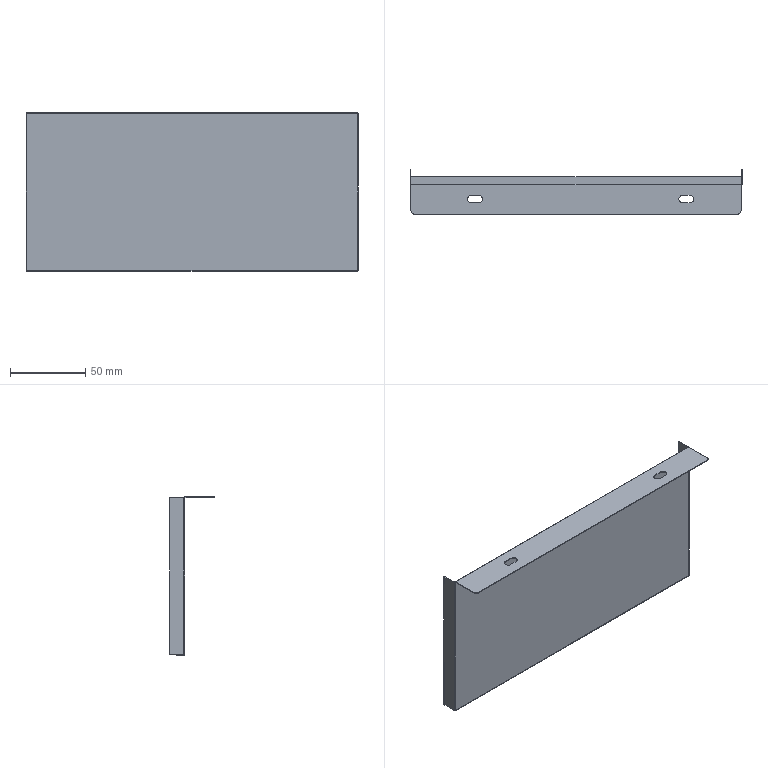Part | SolidWorks | features EdgeFlange 1, Fillet 1, FlatPattern 1, ICE 1, SMBaseFlange 1, SheetMetal 1 | 1 solid | 48 faces | box 220 x 29.5 x 105 mm | volume 15122 mm3 | plane 30 | cylinder 14 | spline 4 | commonest cylinder face diameters 5 x6 0.2 x4 1.2 x4
STEP:
#1=CARTESIAN_POINT('',(0.6,-0.5,0.6));
#2=VERTEX_POINT('',#1);
#3=CARTESIAN_POINT('',(219.4,-0.5,0.6));
#4=VERTEX_POINT('',#3);
#5=CARTESIAN_POINT('',(0.5707,-0.5,0.6));
#6=DIRECTION('',(1.,0.,0.));
#7=VECTOR('',#6,1000.);
#8=LINE('',#5,#7);
#9=EDGE_CURVE('',#2,#4,#8,.T.);
#10=ORIENTED_EDGE('',*,*,#9,.T.);
#11=CARTESIAN_POINT('',(219.4,-0.5,104.4));
#12=VERTEX_POINT('',#11);
#13=CARTESIAN_POINT('',(219.4,-0.5,0.5707));
#14=DIRECTION('',(0.,0.,1.));
#15=VECTOR('',#14,1000.);
#16=LINE('',#13,#15);
#17=EDGE_CURVE('',#4,#12,#16,.T.);
#18=ORIENTED_EDGE('',*,*,#17,.T.);
#19=CARTESIAN_POINT('',(0.6,-0.5,104.4));
#20=VERTEX_POINT('',#19);
#21=CARTESIAN_POINT('',(0.6,-0.5,104.4));
#22=DIRECTION('',(1.,0.,0.));
#23=VECTOR('',#22,1000.);
#24=LINE('',#21,#23);
#25=EDGE_CURVE('',#20,#12,#24,.T.);
#26=ORIENTED_EDGE('',*,*,#25,.F.);
#27=CARTESIAN_POINT('',(0.6,-0.5,104.4));
#28=DIRECTION('',(0.,0.,-1.));
#29=VECTOR('',#28,1000.);
#30=LINE('',#27,#29);
#31=EDGE_CURVE('',#20,#2,#30,.T.);
#32=ORIENTED_EDGE('',*,*,#31,.T.);
#33=EDGE_LOOP('',(#10,#18,#26,#32));
#34=FACE_OUTER_BOUND('',#33,.T.);
#35=CARTESIAN_POINT('',(0.,-0.5,105.));
#36=DIRECTION('',(0.,1.,0.));
#37=DIRECTION('',(0.,0.,1.));
#38=AXIS2_PLACEMENT_3D('',#35,#36,#37);
#39=PLANE('',#38);
#40=ADVANCED_FACE('',(#34),#39,.F.);
#41=CARTESIAN_POINT('',(219.4,0.,0.6));
#42=VERTEX_POINT('',#41);
#43=CARTESIAN_POINT('',(219.4,0.,104.4));
#44=VERTEX_POINT('',#43);
#45=CARTESIAN_POINT('',(219.4,0.,0.5707));
#46=DIRECTION('',(0.,0.,1.));
#47=VECTOR('',#46,1000.);
#48=LINE('',#45,#47);
#49=EDGE_CURVE('',#42,#44,#48,.T.);
#50=ORIENTED_EDGE('',*,*,#49,.F.);
#51=CARTESIAN_POINT('',(0.6,0.,0.6));
#52=VERTEX_POINT('',#51);
#53=CARTESIAN_POINT('',(0.5707,0.,0.6));
#54=DIRECTION('',(1.,0.,0.));
#55=VECTOR('',#54,1000.);
#56=LINE('',#53,#55);
#57=EDGE_CURVE('',#52,#42,#56,.T.);
#58=ORIENTED_EDGE('',*,*,#57,.F.);
#59=CARTESIAN_POINT('',(0.6,0.,104.4));
#60=VERTEX_POINT('',#59);
#61=CARTESIAN_POINT('',(0.6,0.,104.4));
#62=DIRECTION('',(0.,0.,-1.));
#63=VECTOR('',#62,1000.);
#64=LINE('',#61,#63);
#65=EDGE_CURVE('',#60,#52,#64,.T.);
#66=ORIENTED_EDGE('',*,*,#65,.F.);
#67=CARTESIAN_POINT('',(0.6,0.,104.4));
#68=DIRECTION('',(1.,0.,0.));
#69=VECTOR('',#68,1000.);
#70=LINE('',#67,#69);
#71=EDGE_CURVE('',#60,#44,#70,.T.);
#72=ORIENTED_EDGE('',*,*,#71,.T.);
#73=EDGE_LOOP('',(#50,#58,#66,#72));
#74=FACE_OUTER_BOUND('',#73,.T.);
#75=CARTESIAN_POINT('',(0.,0.,105.));
#76=DIRECTION('',(0.,1.,0.));
#77=DIRECTION('',(0.,0.,1.));
#78=AXIS2_PLACEMENT_3D('',#75,#76,#77);
#79=PLANE('',#78);
#80=ADVANCED_FACE('',(#74),#79,.T.);
#81=CARTESIAN_POINT('',(0.,0.1,0.5707));
#82=VERTEX_POINT('',#81);
#83=CARTESIAN_POINT('',(0.5,0.1,0.5707));
#84=VERTEX_POINT('',#83);
#85=CARTESIAN_POINT('',(0.5,0.1,0.5707));
#86=DIRECTION('',(1.,0.,0.));
#87=VECTOR('',#86,1000.);
#88=LINE('',#85,#87);
#89=EDGE_CURVE('',#82,#84,#88,.T.);
#90=ORIENTED_EDGE('',*,*,#89,.T.);
#91=CARTESIAN_POINT('',(0.6,0.,0.6));
#92=CARTESIAN_POINT('',(0.5738,0.,0.5951));
#93=CARTESIAN_POINT('',(0.5478,0.01078,0.5902));
#94=CARTESIAN_POINT('',(0.5108,0.0478,0.5805));
#95=CARTESIAN_POINT('',(0.5,0.07382,0.5756));
#96=CARTESIAN_POINT('',(0.5,0.1,0.5707));
#97=B_SPLINE_CURVE_WITH_KNOTS('',3,(#91,#92,#93,#94,#95,#96),.UNSPECIFIED.,.F.,.F.,(4,2,4),(0.,0.5,1.),.UNSPECIFIED.);
#98=EDGE_CURVE('',#52,#84,#97,.T.);
#99=ORIENTED_EDGE('',*,*,#98,.F.);
#100=CARTESIAN_POINT('',(0.6,0.,0.6));
#101=DIRECTION('',(0.,-1.,0.));
#102=VECTOR('',#101,1000.);
#103=LINE('',#100,#102);
#104=EDGE_CURVE('',#52,#2,#103,.T.);
#105=ORIENTED_EDGE('',*,*,#104,.T.);
#106=CARTESIAN_POINT('',(0.6,-0.5,0.6));
#107=CARTESIAN_POINT('',(0.4429,-0.5,0.5951));
#108=CARTESIAN_POINT('',(0.2868,-0.4353,0.5902));
#109=CARTESIAN_POINT('',(0.06466,-0.2132,0.5805));
#110=CARTESIAN_POINT('',(0.,-0.05708,0.5756));
#111=CARTESIAN_POINT('',(0.,0.1,0.5707));
#112=B_SPLINE_CURVE_WITH_KNOTS('',3,(#106,#107,#108,#109,#110,#111),.UNSPECIFIED.,.F.,.F.,(4,2,4),(0.,0.5,1.),.UNSPECIFIED.);
#113=EDGE_CURVE('',#2,#82,#112,.T.);
#114=ORIENTED_EDGE('',*,*,#113,.T.);
#115=EDGE_LOOP('',(#90,#99,#105,#114));
#116=FACE_OUTER_BOUND('',#115,.T.);
#117=CARTESIAN_POINT('',(0.6,-0.505,0.6));
#118=CARTESIAN_POINT('',(0.5208,-0.505,0.5976));
#119=CARTESIAN_POINT('',(0.4416,-0.4893,0.5951));
#120=CARTESIAN_POINT('',(0.2953,-0.4286,0.5902));
#121=CARTESIAN_POINT('',(0.2282,-0.3838,0.5878));
#122=CARTESIAN_POINT('',(0.1162,-0.2718,0.5829));
#123=CARTESIAN_POINT('',(0.07136,-0.2047,0.5805));
#124=CARTESIAN_POINT('',(0.01075,-0.05836,0.5756));
#125=CARTESIAN_POINT('',(-0.005,0.02079,0.5732));
#126=CARTESIAN_POINT('',(-0.005,0.1,0.5707));
#127=CARTESIAN_POINT('',(0.6,-0.5,0.6));
#128=CARTESIAN_POINT('',(0.5214,-0.5,0.5976));
#129=CARTESIAN_POINT('',(0.443,-0.4844,0.5951));
#130=CARTESIAN_POINT('',(0.2978,-0.4243,0.5902));
#131=CARTESIAN_POINT('',(0.2313,-0.3798,0.5878));
#132=CARTESIAN_POINT('',(0.1202,-0.2687,0.5829));
#133=CARTESIAN_POINT('',(0.07573,-0.2022,0.5805));
#134=CARTESIAN_POINT('',(0.01562,-0.05705,0.5756));
#135=CARTESIAN_POINT('',(0.,0.02145,0.5732));
#136=CARTESIAN_POINT('',(0.,0.1,0.5707));
#137=CARTESIAN_POINT('',(0.6,0.,0.6));
#138=CARTESIAN_POINT('',(0.5869,0.,0.5976));
#139=CARTESIAN_POINT('',(0.5738,0.002603,0.5951));
#140=CARTESIAN_POINT('',(0.5496,0.01262,0.5902));
#141=CARTESIAN_POINT('',(0.5385,0.02003,0.5878));
#142=CARTESIAN_POINT('',(0.52,0.03855,0.5829));
#143=CARTESIAN_POINT('',(0.5126,0.04964,0.5805));
#144=CARTESIAN_POINT('',(0.5026,0.07383,0.5756));
#145=CARTESIAN_POINT('',(0.5,0.08691,0.5732));
#146=CARTESIAN_POINT('',(0.5,0.1,0.5707));
#147=CARTESIAN_POINT('',(0.6,0.00505,0.6));
#148=CARTESIAN_POINT('',(0.5876,0.00505,0.5976));
#149=CARTESIAN_POINT('',(0.5751,0.007521,0.5951));
#150=CARTESIAN_POINT('',(0.5522,0.01703,0.5902));
#151=CARTESIAN_POINT('',(0.5416,0.02407,0.5878));
#152=CARTESIAN_POINT('',(0.5241,0.04165,0.5829));
#153=CARTESIAN_POINT('',(0.517,0.05218,0.5805));
#154=CARTESIAN_POINT('',(0.5075,0.07515,0.5756));
#155=CARTESIAN_POINT('',(0.505,0.08757,0.5732));
#156=CARTESIAN_POINT('',(0.505,0.1,0.5707));
#157=B_SPLINE_SURFACE_WITH_KNOTS('',1,3,((#117,#118,#119,#120,#121,#122,#123,#124,#125,#126),(#127,#128,#129,#130,#131,#132,#133,#134,#135,#136),(#137,#138,#139,#140,#141,#142,#143,#144,#145,#146),(#147,#148,#149,#150,#151,#152,#153,#154,#155,#156)),.UNSPECIFIED.,.F.,.F.,.F.,(2,1,1,2),(4,2,2,2,4),(-0.01,0.,1.,1.01),(0.,0.25,0.5,0.75,1.),.UNSPECIFIED.);
#158=ADVANCED_FACE('',(#116),#157,.F.);
#159=ORIENTED_EDGE('',*,*,#31,.F.);
#160=CARTESIAN_POINT('',(0.,0.1,104.4));
#161=VERTEX_POINT('',#160);
#162=CARTESIAN_POINT('',(0.6,0.1,104.4));
#163=DIRECTION('',(0.,0.,1.));
#164=DIRECTION('',(1.,0.,0.));
#165=AXIS2_PLACEMENT_3D('',#162,#163,#164);
#166=CIRCLE('',#165,0.6);
#167=EDGE_CURVE('',#161,#20,#166,.T.);
#168=ORIENTED_EDGE('',*,*,#167,.F.);
#169=CARTESIAN_POINT('',(0.,0.1,0.));
#170=DIRECTION('',(0.,0.,-1.));
#171=VECTOR('',#170,1000.);
#172=LINE('',#169,#171);
#173=EDGE_CURVE('',#161,#82,#172,.T.);
#174=ORIENTED_EDGE('',*,*,#173,.T.);
#175=ORIENTED_EDGE('',*,*,#113,.F.);
#176=EDGE_LOOP('',(#159,#168,#174,#175));
#177=FACE_OUTER_BOUND('',#176,.T.);
#178=CARTESIAN_POINT('',(0.6,0.1,104.4));
#179=DIRECTION('',(0.,0.,1.));
#180=DIRECTION('',(-1.,0.,0.));
#181=AXIS2_PLACEMENT_3D('',#178,#179,#180);
#182=CYLINDRICAL_SURFACE('',#181,0.6);
#183=ADVANCED_FACE('',(#177),#182,.T.);
#184=CARTESIAN_POINT('',(0.5,0.1,104.4));
#185=VERTEX_POINT('',#184);
#186=CARTESIAN_POINT('',(0.6,0.1,104.4));
#187=DIRECTION('',(0.,0.,1.));
#188=DIRECTION('',(1.,0.,0.));
#189=AXIS2_PLACEMENT_3D('',#186,#187,#188);
#190=CIRCLE('',#189,0.1);
#191=EDGE_CURVE('',#185,#60,#190,.T.);
#192=ORIENTED_EDGE('',*,*,#191,.F.);
#193=CARTESIAN_POINT('',(0.5,0.1,104.4));
#194=DIRECTION('',(1.,0.,0.));
#195=VECTOR('',#194,1000.);
#196=LINE('',#193,#195);
#197=EDGE_CURVE('',#161,#185,#196,.T.);
#198=ORIENTED_EDGE('',*,*,#197,.F.);
#199=ORIENTED_EDGE('',*,*,#167,.T.);
#200=CARTESIAN_POINT('',(0.6,0.,104.4));
#201=DIRECTION('',(0.,-1.,0.));
#202=VECTOR('',#201,1000.);
#203=LINE('',#200,#202);
#204=EDGE_CURVE('',#60,#20,#203,.T.);
#205=ORIENTED_EDGE('',*,*,#204,.F.);
#206=EDGE_LOOP('',(#192,#198,#199,#205));
#207=FACE_OUTER_BOUND('',#206,.T.);
#208=CARTESIAN_POINT('',(0.6,0.1,104.4));
#209=DIRECTION('',(0.,0.,-1.));
#210=DIRECTION('',(-1.,0.,0.));
#211=AXIS2_PLACEMENT_3D('',#208,#209,#210);
#212=PLANE('',#211);
#213=ADVANCED_FACE('',(#207),#212,.F.);
#214=ORIENTED_EDGE('',*,*,#65,.T.);
#215=ORIENTED_EDGE('',*,*,#98,.T.);
#216=CARTESIAN_POINT('',(0.5,0.1,0.));
#217=DIRECTION('',(0.,0.,1.));
#218=VECTOR('',#217,1000.);
#219=LINE('',#216,#218);
#220=EDGE_CURVE('',#84,#185,#219,.T.);
#221=ORIENTED_EDGE('',*,*,#220,.T.);
#222=ORIENTED_EDGE('',*,*,#191,.T.);
#223=EDGE_LOOP('',(#214,#215,#221,#222));
#224=FACE_OUTER_BOUND('',#223,.T.);
#225=CARTESIAN_POINT('',(0.6,0.1,104.4));
#226=DIRECTION('',(0.,0.,1.));
#227=DIRECTION('',(-1.,0.,0.));
#228=AXIS2_PLACEMENT_3D('',#225,#226,#227);
#229=CYLINDRICAL_SURFACE('',#228,0.1);
#230=ADVANCED_FACE('',(#224),#229,.F.);
#231=CARTESIAN_POINT('',(0.,9.5,0.5707));
#232=VERTEX_POINT('',#231);
#233=CARTESIAN_POINT('',(0.,0.,0.5707));
#234=DIRECTION('',(0.,1.,0.));
#235=VECTOR('',#234,1000.);
#236=LINE('',#233,#235);
#237=EDGE_CURVE('',#82,#232,#236,.T.);
#238=ORIENTED_EDGE('',*,*,#237,.T.);
#239=CARTESIAN_POINT('',(0.5,9.5,0.5707));
#240=VERTEX_POINT('',#239);
#241=CARTESIAN_POINT('',(0.5,9.5,0.5707));
#242=DIRECTION('',(1.,0.,0.));
#243=VECTOR('',#242,1000.);
#244=LINE('',#241,#243);
#245=EDGE_CURVE('',#232,#240,#244,.T.);
#246=ORIENTED_EDGE('',*,*,#245,.T.);
#247=CARTESIAN_POINT('',(0.5,0.,0.5707));
#248=DIRECTION('',(0.,1.,0.));
#249=VECTOR('',#248,1000.);
#250=LINE('',#247,#249);
#251=EDGE_CURVE('',#84,#240,#250,.T.);
#252=ORIENTED_EDGE('',*,*,#251,.F.);
#253=ORIENTED_EDGE('',*,*,#89,.F.);
#254=EDGE_LOOP('',(#238,#246,#252,#253));
#255=FACE_OUTER_BOUND('',#254,.T.);
#256=CARTESIAN_POINT('',(0.5,0.,0.5707));
#257=DIRECTION('',(0.,0.,-1.));
#258=DIRECTION('',(0.,1.,0.));
#259=AXIS2_PLACEMENT_3D('',#256,#257,#258);
#260=PLANE('',#259);
#261=ADVANCED_FACE('',(#255),#260,.T.);
#262=ORIENTED_EDGE('',*,*,#237,.F.);
#263=ORIENTED_EDGE('',*,*,#173,.F.);
#264=CARTESIAN_POINT('',(0.,9.5,104.4));
#265=VERTEX_POINT('',#264);
#266=CARTESIAN_POINT('',(0.,0.,104.4));
#267=DIRECTION('',(0.,1.,0.));
#268=VECTOR('',#267,1000.);
#269=LINE('',#266,#268);
#270=EDGE_CURVE('',#161,#265,#269,.T.);
#271=ORIENTED_EDGE('',*,*,#270,.T.);
#272=CARTESIAN_POINT('',(0.,9.5,0.));
#273=DIRECTION('',(0.,0.,-1.));
#274=VECTOR('',#273,1000.);
#275=LINE('',#272,#274);
#276=EDGE_CURVE('',#265,#232,#275,.T.);
#277=ORIENTED_EDGE('',*,*,#276,.T.);
#278=EDGE_LOOP('',(#262,#263,#271,#277));
#279=FACE_OUTER_BOUND('',#278,.T.);
#280=CARTESIAN_POINT('',(0.,0.,0.));
#281=DIRECTION('',(1.,0.,0.));
#282=DIRECTION('',(0.,1.,0.));
#283=AXIS2_PLACEMENT_3D('',#280,#281,#282);
#284=PLANE('',#283);
#285=ADVANCED_FACE('',(#279),#284,.F.);
#286=ORIENTED_EDGE('',*,*,#220,.F.);
#287=ORIENTED_EDGE('',*,*,#251,.T.);
#288=CARTESIAN_POINT('',(0.5,9.5,104.4));
#289=VERTEX_POINT('',#288);
#290=CARTESIAN_POINT('',(0.5,9.5,0.));
#291=DIRECTION('',(0.,0.,-1.));
#292=VECTOR('',#291,1000.);
#293=LINE('',#290,#292);
#294=EDGE_CURVE('',#289,#240,#293,.T.);
#295=ORIENTED_EDGE('',*,*,#294,.F.);
#296=CARTESIAN_POINT('',(0.5,0.,104.4));
#297=DIRECTION('',(0.,1.,0.));
#298=VECTOR('',#297,1000.);
#299=LINE('',#296,#298);
#300=EDGE_CURVE('',#185,#289,#299,.T.);
#301=ORIENTED_EDGE('',*,*,#300,.F.);
#302=EDGE_LOOP('',(#286,#287,#295,#301));
#303=FACE_OUTER_BOUND('',#302,.T.);
#304=CARTESIAN_POINT('',(0.5,0.,0.));
#305=DIRECTION('',(1.,0.,0.));
#306=DIRECTION('',(0.,1.,0.));
#307=AXIS2_PLACEMENT_3D('',#304,#305,#306);
#308=PLANE('',#307);
#309=ADVANCED_FACE('',(#303),#308,.T.);
#310=ORIENTED_EDGE('',*,*,#245,.F.);
#311=ORIENTED_EDGE('',*,*,#276,.F.);
#312=CARTESIAN_POINT('',(0.,9.5,104.4));
#313=DIRECTION('',(1.,0.,0.));
#314=VECTOR('',#313,1000.);
#315=LINE('',#312,#314);
#316=EDGE_CURVE('',#265,#289,#315,.T.);
#317=ORIENTED_EDGE('',*,*,#316,.T.);
#318=ORIENTED_EDGE('',*,*,#294,.T.);
#319=EDGE_LOOP('',(#310,#311,#317,#318));
#320=FACE_OUTER_BOUND('',#319,.T.);
#321=CARTESIAN_POINT('',(0.,9.5,0.));
#322=DIRECTION('',(0.,-1.,0.));
#323=DIRECTION('',(1.,0.,0.));
#324=AXIS2_PLACEMENT_3D('',#321,#322,#323);
#325=PLANE('',#324);
#326=ADVANCED_FACE('',(#320),#325,.F.);
#327=ORIENTED_EDGE('',*,*,#316,.F.);
#328=ORIENTED_EDGE('',*,*,#270,.F.);
#329=ORIENTED_EDGE('',*,*,#197,.T.);
#330=ORIENTED_EDGE('',*,*,#300,.T.);
#331=EDGE_LOOP('',(#327,#328,#329,#330));
#332=FACE_OUTER_BOUND('',#331,.T.);
#333=CARTESIAN_POINT('',(0.5,0.,104.4));
#334=DIRECTION('',(0.,0.,-1.));
#335=DIRECTION('',(0.,1.,0.));
#336=AXIS2_PLACEMENT_3D('',#333,#334,#335);
#337=PLANE('',#336);
#338=ADVANCED_FACE('',(#332),#337,.F.);
#339=CARTESIAN_POINT('',(219.4,-0.6,105.));
#340=VERTEX_POINT('',#339);
#341=CARTESIAN_POINT('',(219.4,-0.6,104.5));
#342=VERTEX_POINT('',#341);
#343=CARTESIAN_POINT('',(219.4,-0.6,104.5));
#344=DIRECTION('',(0.,0.,-1.));
#345=VECTOR('',#344,1000.);
#346=LINE('',#343,#345);
#347=EDGE_CURVE('',#340,#342,#346,.T.);
#348=ORIENTED_EDGE('',*,*,#347,.T.);
#349=CARTESIAN_POINT('',(219.4,-0.6,104.4));
#350=DIRECTION('',(1.,0.,0.));
#351=DIRECTION('',(0.,0.,1.));
#352=AXIS2_PLACEMENT_3D('',#349,#350,#351);
#353=CIRCLE('',#352,0.1);
#354=EDGE_CURVE('',#12,#342,#353,.T.);
#355=ORIENTED_EDGE('',*,*,#354,.F.);
#356=CARTESIAN_POINT('',(219.4,-0.5,104.4));
#357=DIRECTION('',(0.,1.,0.));
#358=VECTOR('',#357,1000.);
#359=LINE('',#356,#358);
#360=EDGE_CURVE('',#12,#44,#359,.T.);
#361=ORIENTED_EDGE('',*,*,#360,.T.);
#362=CARTESIAN_POINT('',(219.4,-0.6,104.4));
#363=DIRECTION('',(1.,0.,0.));
#364=DIRECTION('',(0.,0.,1.));
#365=AXIS2_PLACEMENT_3D('',#362,#363,#364);
#366=CIRCLE('',#365,0.6);
#367=EDGE_CURVE('',#44,#340,#366,.T.);
#368=ORIENTED_EDGE('',*,*,#367,.T.);
#369=EDGE_LOOP('',(#348,#355,#361,#368));
#370=FACE_OUTER_BOUND('',#369,.T.);
#371=CARTESIAN_POINT('',(219.4,-0.6,104.4));
#372=DIRECTION('',(1.,0.,0.));
#373=DIRECTION('',(0.,0.,-1.));
#374=AXIS2_PLACEMENT_3D('',#371,#372,#373);
#375=PLANE('',#374);
#376=ADVANCED_FACE('',(#370),#375,.T.);
#377=ORIENTED_EDGE('',*,*,#71,.F.);
#378=CARTESIAN_POINT('',(0.6,-0.6,105.));
#379=VERTEX_POINT('',#378);
#380=CARTESIAN_POINT('',(0.6,-0.6,104.4));
#381=DIRECTION('',(-1.,0.,0.));
#382=DIRECTION('',(0.,0.,1.));
#383=AXIS2_PLACEMENT_3D('',#380,#381,#382);
#384=CIRCLE('',#383,0.6);
#385=EDGE_CURVE('',#379,#60,#384,.T.);
#386=ORIENTED_EDGE('',*,*,#385,.F.);
#387=CARTESIAN_POINT('',(220.,-0.6,105.));
#388=DIRECTION('',(1.,0.,0.));
#389=VECTOR('',#388,1000.);
#390=LINE('',#387,#389);
#391=EDGE_CURVE('',#379,#340,#390,.T.);
#392=ORIENTED_EDGE('',*,*,#391,.T.);
#393=ORIENTED_EDGE('',*,*,#367,.F.);
#394=EDGE_LOOP('',(#377,#386,#392,#393));
#395=FACE_OUTER_BOUND('',#394,.T.);
#396=CARTESIAN_POINT('',(0.6,-0.6,104.4));
#397=DIRECTION('',(-1.,0.,0.));
#398=DIRECTION('',(0.,0.,1.));
#399=AXIS2_PLACEMENT_3D('',#396,#397,#398);
#400=CYLINDRICAL_SURFACE('',#399,0.6);
#401=ADVANCED_FACE('',(#395),#400,.T.);
#402=CARTESIAN_POINT('',(0.6,-0.6,104.5));
#403=VERTEX_POINT('',#402);
#404=CARTESIAN_POINT('',(0.6,-0.6,104.4));
#405=DIRECTION('',(-1.,0.,0.));
#406=DIRECTION('',(0.,0.,1.));
#407=AXIS2_PLACEMENT_3D('',#404,#405,#406);
#408=CIRCLE('',#407,0.1);
#409=EDGE_CURVE('',#403,#20,#408,.T.);
#410=ORIENTED_EDGE('',*,*,#409,.F.);
#411=CARTESIAN_POINT('',(0.6,-0.6,104.5));
#412=DIRECTION('',(0.,0.,-1.));
#413=VECTOR('',#412,1000.);
#414=LINE('',#411,#413);
#415=EDGE_CURVE('',#379,#403,#414,.T.);
#416=ORIENTED_EDGE('',*,*,#415,.F.);
#417=ORIENTED_EDGE('',*,*,#385,.T.);
#418=ORIENTED_EDGE('',*,*,#204,.T.);
#419=EDGE_LOOP('',(#410,#416,#417,#418));
#420=FACE_OUTER_BOUND('',#419,.T.);
#421=CARTESIAN_POINT('',(0.6,-0.6,104.4));
#422=DIRECTION('',(1.,0.,0.));
#423=DIRECTION('',(0.,0.,-1.));
#424=AXIS2_PLACEMENT_3D('',#421,#422,#423);
#425=PLANE('',#424);
#426=ADVANCED_FACE('',(#420),#425,.F.);
#427=ORIENTED_EDGE('',*,*,#25,.T.);
#428=ORIENTED_EDGE('',*,*,#354,.T.);
#429=CARTESIAN_POINT('',(220.,-0.6,104.5));
#430=DIRECTION('',(-1.,0.,0.));
#431=VECTOR('',#430,1000.);
#432=LINE('',#429,#431);
#433=EDGE_CURVE('',#342,#403,#432,.T.);
#434=ORIENTED_EDGE('',*,*,#433,.T.);
#435=ORIENTED_EDGE('',*,*,#409,.T.);
#436=EDGE_LOOP('',(#427,#428,#434,#435));
#437=FACE_OUTER_BOUND('',#436,.T.);
#438=CARTESIAN_POINT('',(0.6,-0.6,104.4));
#439=DIRECTION('',(-1.,0.,0.));
#440=DIRECTION('',(0.,0.,1.));
#441=AXIS2_PLACEMENT_3D('',#438,#439,#440);
#442=CYLINDRICAL_SURFACE('',#441,0.1);
#443=ADVANCED_FACE('',(#437),#442,.F.);
#444=CARTESIAN_POINT('',(219.4,-17.5,105.));
#445=VERTEX_POINT('',#444);
#446=CARTESIAN_POINT('',(219.4,-0.5,105.));
#447=DIRECTION('',(0.,-1.,0.));
#448=VECTOR('',#447,1000.);
#449=LINE('',#446,#448);
#450=EDGE_CURVE('',#340,#445,#449,.T.);
#451=ORIENTED_EDGE('',*,*,#450,.T.);
#452=CARTESIAN_POINT('',(219.4,-17.5,104.5));
#453=VERTEX_POINT('',#452);
#454=CARTESIAN_POINT('',(219.4,-17.5,104.5));
#455=DIRECTION('',(0.,0.,-1.));
#456=VECTOR('',#455,1000.);
#457=LINE('',#454,#456);
#458=EDGE_CURVE('',#445,#453,#457,.T.);
#459=ORIENTED_EDGE('',*,*,#458,.T.);
#460=CARTESIAN_POINT('',(219.4,-20.,104.5));
#461=DIRECTION('',(0.,-1.,0.));
#462=VECTOR('',#461,1000.);
#463=LINE('',#460,#462);
#464=EDGE_CURVE('',#342,#453,#463,.T.);
#465=ORIENTED_EDGE('',*,*,#464,.F.);
#466=ORIENTED_EDGE('',*,*,#347,.F.);
#467=EDGE_LOOP('',(#451,#459,#465,#466));
#468=FACE_OUTER_BOUND('',#467,.T.);
#469=CARTESIAN_POINT('',(219.4,-0.5,104.5));
#470=DIRECTION('',(1.,0.,0.));
#471=DIRECTION('',(0.,0.,-1.));
#472=AXIS2_PLACEMENT_3D('',#469,#470,#471);
#473=PLANE('',#472);
#474=ADVANCED_FACE('',(#468),#473,.T.);
#475=CARTESIAN_POINT('',(185.6,-12.5,105.));
#476=VERTEX_POINT('',#475);
#477=CARTESIAN_POINT('',(180.6,-12.5,105.));
#478=VERTEX_POINT('',#477);
#479=CARTESIAN_POINT('',(220.,-12.5,105.));
#480=DIRECTION('',(-1.,0.,0.));
#481=VECTOR('',#480,1000.);
#482=LINE('',#479,#481);
#483=EDGE_CURVE('',#476,#478,#482,.T.);
#484=ORIENTED_EDGE('',*,*,#483,.T.);
#485=CARTESIAN_POINT('',(180.6,-7.5,105.));
#486=VERTEX_POINT('',#485);
#487=CARTESIAN_POINT('',(180.6,-10.,105.));
#488=DIRECTION('',(0.,0.,-1.));
#489=DIRECTION('',(0.,1.,0.));
#490=AXIS2_PLACEMENT_3D('',#487,#488,#489);
#491=CIRCLE('',#490,2.5);
#492=EDGE_CURVE('',#478,#486,#491,.T.);
#493=ORIENTED_EDGE('',*,*,#492,.T.);
#494=CARTESIAN_POINT('',(185.6,-7.5,105.));
#495=VERTEX_POINT('',#494);
#496=CARTESIAN_POINT('',(220.,-7.5,105.));
#497=DIRECTION('',(1.,0.,0.));
#498=VECTOR('',#497,1000.);
#499=LINE('',#496,#498);
#500=EDGE_CURVE('',#486,#495,#499,.T.);
#501=ORIENTED_EDGE('',*,*,#500,.T.);
#502=CARTESIAN_POINT('',(185.6,-10.,105.));
#503=DIRECTION('',(0.,0.,-1.));
#504=DIRECTION('',(0.,1.,0.));
#505=AXIS2_PLACEMENT_3D('',#502,#503,#504);
#506=CIRCLE('',#505,2.5);
#507=EDGE_CURVE('',#495,#476,#506,.T.);
#508=ORIENTED_EDGE('',*,*,#507,.T.);
#509=EDGE_LOOP('',(#484,#493,#501,#508));
#510=FACE_BOUND('',#509,.T.);
#511=CARTESIAN_POINT('',(45.6,-12.5,105.));
#512=VERTEX_POINT('',#511);
#513=CARTESIAN_POINT('',(40.6,-12.5,105.));
#514=VERTEX_POINT('',#513);
#515=CARTESIAN_POINT('',(220.,-12.5,105.));
#516=DIRECTION('',(-1.,0.,0.));
#517=VECTOR('',#516,1000.);
#518=LINE('',#515,#517);
#519=EDGE_CURVE('',#512,#514,#518,.T.);
#520=ORIENTED_EDGE('',*,*,#519,.T.);
#521=CARTESIAN_POINT('',(40.6,-7.5,105.));
#522=VERTEX_POINT('',#521);
#523=CARTESIAN_POINT('',(40.6,-10.,105.));
#524=DIRECTION('',(0.,0.,-1.));
#525=DIRECTION('',(0.,1.,0.));
#526=AXIS2_PLACEMENT_3D('',#523,#524,#525);
#527=CIRCLE('',#526,2.5);
#528=EDGE_CURVE('',#514,#522,#527,.T.);
#529=ORIENTED_EDGE('',*,*,#528,.T.);
#530=CARTESIAN_POINT('',(45.6,-7.5,105.));
#531=VERTEX_POINT('',#530);
#532=CARTESIAN_POINT('',(220.,-7.5,105.));
#533=DIRECTION('',(1.,0.,0.));
#534=VECTOR('',#533,1000.);
#535=LINE('',#532,#534);
#536=EDGE_CURVE('',#522,#531,#535,.T.);
#537=ORIENTED_EDGE('',*,*,#536,.T.);
#538=CARTESIAN_POINT('',(45.6,-10.,105.));
#539=DIRECTION('',(0.,0.,-1.));
#540=DIRECTION('',(0.,1.,0.));
#541=AXIS2_PLACEMENT_3D('',#538,#539,#540);
#542=CIRCLE('',#541,2.5);
#543=EDGE_CURVE('',#531,#512,#542,.T.);
#544=ORIENTED_EDGE('',*,*,#543,.T.);
#545=EDGE_LOOP('',(#520,#529,#537,#544));
#546=FACE_BOUND('',#545,.T.);
#547=CARTESIAN_POINT('',(216.9,-20.,105.));
#548=VERTEX_POINT('',#547);
#549=CARTESIAN_POINT('',(3.1,-20.,105.));
#550=VERTEX_POINT('',#549);
#551=CARTESIAN_POINT('',(220.,-20.,105.));
#552=DIRECTION('',(-1.,0.,0.));
#553=VECTOR('',#552,1000.);
#554=LINE('',#551,#553);
#555=EDGE_CURVE('',#548,#550,#554,.T.);
#556=ORIENTED_EDGE('',*,*,#555,.F.);
#557=CARTESIAN_POINT('',(216.9,-17.5,105.));
#558=DIRECTION('',(0.,0.,1.));
#559=DIRECTION('',(0.,1.,0.));
#560=AXIS2_PLACEMENT_3D('',#557,#558,#559);
#561=CIRCLE('',#560,2.5);
#562=EDGE_CURVE('',#548,#445,#561,.T.);
#563=ORIENTED_EDGE('',*,*,#562,.T.);
#564=ORIENTED_EDGE('',*,*,#450,.F.);
#565=ORIENTED_EDGE('',*,*,#391,.F.);
#566=CARTESIAN_POINT('',(0.6,-17.5,105.));
#567=VERTEX_POINT('',#566);
#568=CARTESIAN_POINT('',(0.6,-20.,105.));
#569=DIRECTION('',(0.,-1.,0.));
#570=VECTOR('',#569,1000.);
#571=LINE('',#568,#570);
#572=EDGE_CURVE('',#379,#567,#571,.T.);
#573=ORIENTED_EDGE('',*,*,#572,.T.);
#574=CARTESIAN_POINT('',(3.1,-17.5,105.));
#575=DIRECTION('',(0.,0.,1.));
#576=DIRECTION('',(0.,1.,0.));
#577=AXIS2_PLACEMENT_3D('',#574,#575,#576);
#578=CIRCLE('',#577,2.5);
#579=EDGE_CURVE('',#567,#550,#578,.T.);
#580=ORIENTED_EDGE('',*,*,#579,.T.);
#581=EDGE_LOOP('',(#556,#563,#564,#565,#573,#580));
#582=FACE_OUTER_BOUND('',#581,.T.);
#583=CARTESIAN_POINT('',(220.,-20.,105.));
#584=DIRECTION('',(0.,0.,-1.));
#585=DIRECTION('',(0.,1.,0.));
#586=AXIS2_PLACEMENT_3D('',#583,#584,#585);
#587=PLANE('',#586);
#588=ADVANCED_FACE('',(#510,#546,#582),#587,.F.);
#589=CARTESIAN_POINT('',(180.6,-12.5,104.5));
#590=VERTEX_POINT('',#589);
#591=CARTESIAN_POINT('',(180.6,-7.5,104.5));
#592=VERTEX_POINT('',#591);
#593=CARTESIAN_POINT('',(180.6,-10.,104.5));
#594=DIRECTION('',(0.,0.,-1.));
#595=DIRECTION('',(0.,1.,0.));
#596=AXIS2_PLACEMENT_3D('',#593,#594,#595);
#597=CIRCLE('',#596,2.5);
#598=EDGE_CURVE('',#590,#592,#597,.T.);
#599=ORIENTED_EDGE('',*,*,#598,.F.);
#600=CARTESIAN_POINT('',(185.6,-12.5,104.5));
#601=VERTEX_POINT('',#600);
#602=CARTESIAN_POINT('',(180.6,-12.5,104.5));
#603=DIRECTION('',(-1.,0.,0.));
#604=VECTOR('',#603,1000.);
#605=LINE('',#602,#604);
#606=EDGE_CURVE('',#601,#590,#605,.T.);
#607=ORIENTED_EDGE('',*,*,#606,.F.);
#608=CARTESIAN_POINT('',(185.6,-7.5,104.5));
#609=VERTEX_POINT('',#608);
#610=CARTESIAN_POINT('',(185.6,-10.,104.5));
#611=DIRECTION('',(0.,0.,-1.));
#612=DIRECTION('',(0.,1.,0.));
#613=AXIS2_PLACEMENT_3D('',#610,#611,#612);
#614=CIRCLE('',#613,2.5);
#615=EDGE_CURVE('',#609,#601,#614,.T.);
#616=ORIENTED_EDGE('',*,*,#615,.F.);
#617=CARTESIAN_POINT('',(180.6,-7.5,104.5));
#618=DIRECTION('',(1.,0.,0.));
#619=VECTOR('',#618,1000.);
#620=LINE('',#617,#619);
#621=EDGE_CURVE('',#592,#609,#620,.T.);
#622=ORIENTED_EDGE('',*,*,#621,.F.);
#623=EDGE_LOOP('',(#599,#607,#616,#622));
#624=FACE_BOUND('',#623,.T.);
#625=CARTESIAN_POINT('',(40.6,-12.5,104.5));
#626=VERTEX_POINT('',#625);
#627=CARTESIAN_POINT('',(40.6,-7.5,104.5));
#628=VERTEX_POINT('',#627);
#629=CARTESIAN_POINT('',(40.6,-10.,104.5));
#630=DIRECTION('',(0.,0.,-1.));
#631=DIRECTION('',(0.,1.,0.));
#632=AXIS2_PLACEMENT_3D('',#629,#630,#631);
#633=CIRCLE('',#632,2.5);
#634=EDGE_CURVE('',#626,#628,#633,.T.);
#635=ORIENTED_EDGE('',*,*,#634,.F.);
#636=CARTESIAN_POINT('',(45.6,-12.5,104.5));
#637=VERTEX_POINT('',#636);
#638=CARTESIAN_POINT('',(40.6,-12.5,104.5));
#639=DIRECTION('',(-1.,0.,0.));
#640=VECTOR('',#639,1000.);
#641=LINE('',#638,#640);
#642=EDGE_CURVE('',#637,#626,#641,.T.);
#643=ORIENTED_EDGE('',*,*,#642,.F.);
#644=CARTESIAN_POINT('',(45.6,-7.5,104.5));
#645=VERTEX_POINT('',#644);
#646=CARTESIAN_POINT('',(45.6,-10.,104.5));
#647=DIRECTION('',(0.,0.,-1.));
#648=DIRECTION('',(0.,1.,0.));
#649=AXIS2_PLACEMENT_3D('',#646,#647,#648);
#650=CIRCLE('',#649,2.5);
#651=EDGE_CURVE('',#645,#637,#650,.T.);
#652=ORIENTED_EDGE('',*,*,#651,.F.);
#653=CARTESIAN_POINT('',(40.6,-7.5,104.5));
#654=DIRECTION('',(1.,0.,0.));
#655=VECTOR('',#654,1000.);
#656=LINE('',#653,#655);
#657=EDGE_CURVE('',#628,#645,#656,.T.);
#658=ORIENTED_EDGE('',*,*,#657,.F.);
#659=EDGE_LOOP('',(#635,#643,#652,#658));
#660=FACE_BOUND('',#659,.T.);
#661=ORIENTED_EDGE('',*,*,#464,.T.);
#662=CARTESIAN_POINT('',(216.9,-20.,104.5));
#663=VERTEX_POINT('',#662);
#664=CARTESIAN_POINT('',(216.9,-17.5,104.5));
#665=DIRECTION('',(0.,0.,-1.));
#666=DIRECTION('',(0.,1.,0.));
#667=AXIS2_PLACEMENT_3D('',#664,#665,#666);
#668=CIRCLE('',#667,2.5);
#669=EDGE_CURVE('',#453,#663,#668,.T.);
#670=ORIENTED_EDGE('',*,*,#669,.T.);
#671=CARTESIAN_POINT('',(3.1,-20.,104.5));
#672=VERTEX_POINT('',#671);
#673=CARTESIAN_POINT('',(220.,-20.,104.5));
#674=DIRECTION('',(-1.,0.,0.));
#675=VECTOR('',#674,1000.);
#676=LINE('',#673,#675);
#677=EDGE_CURVE('',#663,#672,#676,.T.);
#678=ORIENTED_EDGE('',*,*,#677,.T.);
#679=CARTESIAN_POINT('',(0.6,-17.5,104.5));
#680=VERTEX_POINT('',#679);
#681=CARTESIAN_POINT('',(3.1,-17.5,104.5));
#682=DIRECTION('',(0.,0.,-1.));
#683=DIRECTION('',(0.,1.,0.));
#684=AXIS2_PLACEMENT_3D('',#681,#682,#683);
#685=CIRCLE('',#684,2.5);
#686=EDGE_CURVE('',#672,#680,#685,.T.);
#687=ORIENTED_EDGE('',*,*,#686,.T.);
#688=CARTESIAN_POINT('',(0.6,-0.5,104.5));
#689=DIRECTION('',(0.,-1.,0.));
#690=VECTOR('',#689,1000.);
#691=LINE('',#688,#690);
#692=EDGE_CURVE('',#403,#680,#691,.T.);
#693=ORIENTED_EDGE('',*,*,#692,.F.);
#694=ORIENTED_EDGE('',*,*,#433,.F.);
#695=EDGE_LOOP('',(#661,#670,#678,#687,#693,#694));
#696=FACE_OUTER_BOUND('',#695,.T.);
#697=CARTESIAN_POINT('',(220.,-20.,104.5));
#698=DIRECTION('',(0.,0.,-1.));
#699=DIRECTION('',(0.,1.,0.));
#700=AXIS2_PLACEMENT_3D('',#697,#698,#699);
#701=PLANE('',#700);
#702=ADVANCED_FACE('',(#624,#660,#696),#701,.T.);
#703=ORIENTED_EDGE('',*,*,#677,.F.);
#704=CARTESIAN_POINT('',(216.9,-20.,105.));
#705=DIRECTION('',(0.,0.,1.));
#706=VECTOR('',#705,1000.);
#707=LINE('',#704,#706);
#708=EDGE_CURVE('',#663,#548,#707,.T.);
#709=ORIENTED_EDGE('',*,*,#708,.T.);
#710=ORIENTED_EDGE('',*,*,#555,.T.);
#711=CARTESIAN_POINT('',(3.1,-20.,104.5));
#712=DIRECTION('',(0.,0.,-1.));
#713=VECTOR('',#712,1000.);
#714=LINE('',#711,#713);
#715=EDGE_CURVE('',#550,#672,#714,.T.);
#716=ORIENTED_EDGE('',*,*,#715,.T.);
#717=EDGE_LOOP('',(#703,#709,#710,#716));
#718=FACE_OUTER_BOUND('',#717,.T.);
#719=CARTESIAN_POINT('',(220.,-20.,105.));
#720=DIRECTION('',(0.,-1.,0.));
#721=DIRECTION('',(0.,0.,-1.));
#722=AXIS2_PLACEMENT_3D('',#719,#720,#721);
#723=PLANE('',#722);
#724=ADVANCED_FACE('',(#718),#723,.T.);
#725=ORIENTED_EDGE('',*,*,#692,.T.);
#726=CARTESIAN_POINT('',(0.6,-17.5,105.));
#727=DIRECTION('',(0.,0.,1.));
#728=VECTOR('',#727,1000.);
#729=LINE('',#726,#728);
#730=EDGE_CURVE('',#680,#567,#729,.T.);
#731=ORIENTED_EDGE('',*,*,#730,.T.);
#732=ORIENTED_EDGE('',*,*,#572,.F.);
#733=ORIENTED_EDGE('',*,*,#415,.T.);
#734=EDGE_LOOP('',(#725,#731,#732,#733));
#735=FACE_OUTER_BOUND('',#734,.T.);
#736=CARTESIAN_POINT('',(0.6,-0.5,104.5));
#737=DIRECTION('',(1.,0.,0.));
#738=DIRECTION('',(0.,0.,-1.));
#739=AXIS2_PLACEMENT_3D('',#736,#737,#738);
#740=PLANE('',#739);
#741=ADVANCED_FACE('',(#735),#740,.F.);
#742=CARTESIAN_POINT('',(220.,0.1,104.4));
#743=VERTEX_POINT('',#742);
#744=CARTESIAN_POINT('',(219.5,0.1,104.4));
#745=VERTEX_POINT('',#744);
#746=CARTESIAN_POINT('',(219.5,0.1,104.4));
#747=DIRECTION('',(-1.,0.,0.));
#748=VECTOR('',#747,1000.);
#749=LINE('',#746,#748);
#750=EDGE_CURVE('',#743,#745,#749,.T.);
#751=ORIENTED_EDGE('',*,*,#750,.T.);
#752=CARTESIAN_POINT('',(219.4,0.1,104.4));
#753=DIRECTION('',(0.,0.,1.));
#754=DIRECTION('',(-1.,0.,0.));
#755=AXIS2_PLACEMENT_3D('',#752,#753,#754);
#756=CIRCLE('',#755,0.1);
#757=EDGE_CURVE('',#44,#745,#756,.T.);
#758=ORIENTED_EDGE('',*,*,#757,.F.);
#759=ORIENTED_EDGE('',*,*,#360,.F.);
#760=CARTESIAN_POINT('',(219.4,0.1,104.4));
#761=DIRECTION('',(0.,0.,1.));
#762=DIRECTION('',(-1.,0.,0.));
#763=AXIS2_PLACEMENT_3D('',#760,#761,#762);
#764=CIRCLE('',#763,0.6);
#765=EDGE_CURVE('',#12,#743,#764,.T.);
#766=ORIENTED_EDGE('',*,*,#765,.T.);
#767=EDGE_LOOP('',(#751,#758,#759,#766));
#768=FACE_OUTER_BOUND('',#767,.T.);
#769=CARTESIAN_POINT('',(219.4,0.1,104.4));
#770=DIRECTION('',(0.,0.,1.));
#771=DIRECTION('',(1.,0.,0.));
#772=AXIS2_PLACEMENT_3D('',#769,#770,#771);
#773=PLANE('',#772);
#774=ADVANCED_FACE('',(#768),#773,.T.);
#775=ORIENTED_EDGE('',*,*,#17,.F.);
#776=CARTESIAN_POINT('',(220.,0.1,0.5707));
#777=VERTEX_POINT('',#776);
#778=CARTESIAN_POINT('',(220.,0.1,0.5707));
#779=CARTESIAN_POINT('',(220.,-0.05708,0.5756));
#780=CARTESIAN_POINT('',(219.935,-0.2132,0.5805));
#781=CARTESIAN_POINT('',(219.713,-0.4353,0.5902));
#782=CARTESIAN_POINT('',(219.557,-0.5,0.5951));
#783=CARTESIAN_POINT('',(219.4,-0.5,0.6));
#784=B_SPLINE_CURVE_WITH_KNOTS('',3,(#778,#779,#780,#781,#782,#783),.UNSPECIFIED.,.F.,.F.,(4,2,4),(0.,0.5,1.),.UNSPECIFIED.);
#785=EDGE_CURVE('',#777,#4,#784,.T.);
#786=ORIENTED_EDGE('',*,*,#785,.F.);
#787=CARTESIAN_POINT('',(220.,0.1,0.));
#788=DIRECTION('',(0.,0.,-1.));
#789=VECTOR('',#788,1000.);
#790=LINE('',#787,#789);
#791=EDGE_CURVE('',#743,#777,#790,.T.);
#792=ORIENTED_EDGE('',*,*,#791,.F.);
#793=ORIENTED_EDGE('',*,*,#765,.F.);
#794=EDGE_LOOP('',(#775,#786,#792,#793));
#795=FACE_OUTER_BOUND('',#794,.T.);
#796=CARTESIAN_POINT('',(219.4,0.1,0.5707));
#797=DIRECTION('',(0.,0.,-1.));
#798=DIRECTION('',(1.,0.,0.));
#799=AXIS2_PLACEMENT_3D('',#796,#797,#798);
#800=CYLINDRICAL_SURFACE('',#799,0.6);
#801=ADVANCED_FACE('',(#795),#800,.T.);
#802=CARTESIAN_POINT('',(219.5,0.1,0.5707));
#803=VERTEX_POINT('',#802);
#804=CARTESIAN_POINT('',(219.5,0.1,0.5707));
#805=CARTESIAN_POINT('',(219.5,0.07382,0.5756));
#806=CARTESIAN_POINT('',(219.489,0.0478,0.5805));
#807=CARTESIAN_POINT('',(219.452,0.01078,0.5902));
#808=CARTESIAN_POINT('',(219.426,0.,0.5951));
#809=CARTESIAN_POINT('',(219.4,0.,0.6));
#810=B_SPLINE_CURVE_WITH_KNOTS('',3,(#804,#805,#806,#807,#808,#809),.UNSPECIFIED.,.F.,.F.,(4,2,4),(0.,0.5,1.),.UNSPECIFIED.);
#811=EDGE_CURVE('',#803,#42,#810,.T.);
#812=ORIENTED_EDGE('',*,*,#811,.F.);
#813=CARTESIAN_POINT('',(219.5,0.1,0.5707));
#814=DIRECTION('',(-1.,0.,0.));
#815=VECTOR('',#814,1000.);
#816=LINE('',#813,#815);
#817=EDGE_CURVE('',#777,#803,#816,.T.);
#818=ORIENTED_EDGE('',*,*,#817,.F.);
#819=ORIENTED_EDGE('',*,*,#785,.T.);
#820=CARTESIAN_POINT('',(219.4,0.,0.6));
#821=DIRECTION('',(0.,-1.,0.));
#822=VECTOR('',#821,1000.);
#823=LINE('',#820,#822);
#824=EDGE_CURVE('',#42,#4,#823,.T.);
#825=ORIENTED_EDGE('',*,*,#824,.F.);
#826=EDGE_LOOP('',(#812,#818,#819,#825));
#827=FACE_OUTER_BOUND('',#826,.T.);
#828=CARTESIAN_POINT('',(220.005,0.1,0.5707));
#829=CARTESIAN_POINT('',(220.005,0.02079,0.5732));
#830=CARTESIAN_POINT('',(219.989,-0.05836,0.5756));
#831=CARTESIAN_POINT('',(219.929,-0.2047,0.5805));
#832=CARTESIAN_POINT('',(219.884,-0.2718,0.5829));
#833=CARTESIAN_POINT('',(219.772,-0.3838,0.5878));
#834=CARTESIAN_POINT('',(219.705,-0.4286,0.5902));
#835=CARTESIAN_POINT('',(219.558,-0.4893,0.5951));
#836=CARTESIAN_POINT('',(219.479,-0.505,0.5976));
#837=CARTESIAN_POINT('',(219.4,-0.505,0.6));
#838=CARTESIAN_POINT('',(220.,0.1,0.5707));
#839=CARTESIAN_POINT('',(220.,0.02145,0.5732));
#840=CARTESIAN_POINT('',(219.984,-0.05705,0.5756));
#841=CARTESIAN_POINT('',(219.924,-0.2022,0.5805));
#842=CARTESIAN_POINT('',(219.88,-0.2687,0.5829));
#843=CARTESIAN_POINT('',(219.769,-0.3798,0.5878));
#844=CARTESIAN_POINT('',(219.702,-0.4243,0.5902));
#845=CARTESIAN_POINT('',(219.557,-0.4844,0.5951));
#846=CARTESIAN_POINT('',(219.479,-0.5,0.5976));
#847=CARTESIAN_POINT('',(219.4,-0.5,0.6));
#848=CARTESIAN_POINT('',(219.5,0.1,0.5707));
#849=CARTESIAN_POINT('',(219.5,0.08691,0.5732));
#850=CARTESIAN_POINT('',(219.497,0.07383,0.5756));
#851=CARTESIAN_POINT('',(219.487,0.04964,0.5805));
#852=CARTESIAN_POINT('',(219.48,0.03855,0.5829));
#853=CARTESIAN_POINT('',(219.461,0.02003,0.5878));
#854=CARTESIAN_POINT('',(219.45,0.01262,0.5902));
#855=CARTESIAN_POINT('',(219.426,0.002603,0.5951));
#856=CARTESIAN_POINT('',(219.413,0.,0.5976));
#857=CARTESIAN_POINT('',(219.4,0.,0.6));
#858=CARTESIAN_POINT('',(219.495,0.1,0.5707));
#859=CARTESIAN_POINT('',(219.495,0.08757,0.5732));
#860=CARTESIAN_POINT('',(219.492,0.07515,0.5756));
#861=CARTESIAN_POINT('',(219.483,0.05218,0.5805));
#862=CARTESIAN_POINT('',(219.476,0.04165,0.5829));
#863=CARTESIAN_POINT('',(219.458,0.02407,0.5878));
#864=CARTESIAN_POINT('',(219.448,0.01703,0.5902));
#865=CARTESIAN_POINT('',(219.425,0.007521,0.5951));
#866=CARTESIAN_POINT('',(219.412,0.00505,0.5976));
#867=CARTESIAN_POINT('',(219.4,0.00505,0.6));
#868=B_SPLINE_SURFACE_WITH_KNOTS('',1,3,((#828,#829,#830,#831,#832,#833,#834,#835,#836,#837),(#838,#839,#840,#841,#842,#843,#844,#845,#846,#847),(#848,#849,#850,#851,#852,#853,#854,#855,#856,#857),(#858,#859,#860,#861,#862,#863,#864,#865,#866,#867)),.UNSPECIFIED.,.F.,.F.,.F.,(2,1,1,2),(4,2,2,2,4),(-0.01,0.,1.,1.01),(0.,0.25,0.5,0.75,1.),.UNSPECIFIED.);
#869=ADVANCED_FACE('',(#827),#868,.F.);
#870=ORIENTED_EDGE('',*,*,#49,.T.);
#871=ORIENTED_EDGE('',*,*,#757,.T.);
#872=CARTESIAN_POINT('',(219.5,0.1,105.));
#873=DIRECTION('',(0.,0.,-1.));
#874=VECTOR('',#873,1000.);
#875=LINE('',#872,#874);
#876=EDGE_CURVE('',#745,#803,#875,.T.);
#877=ORIENTED_EDGE('',*,*,#876,.T.);
#878=ORIENTED_EDGE('',*,*,#811,.T.);
#879=EDGE_LOOP('',(#870,#871,#877,#878));
#880=FACE_OUTER_BOUND('',#879,.T.);
#881=CARTESIAN_POINT('',(219.4,0.1,0.5707));
#882=DIRECTION('',(0.,0.,-1.));
#883=DIRECTION('',(1.,0.,0.));
#884=AXIS2_PLACEMENT_3D('',#881,#882,#883);
#885=CYLINDRICAL_SURFACE('',#884,0.1);
#886=ADVANCED_FACE('',(#880),#885,.F.);
#887=CARTESIAN_POINT('',(220.,9.5,104.4));
#888=VERTEX_POINT('',#887);
#889=CARTESIAN_POINT('',(220.,0.,104.4));
#890=DIRECTION('',(0.,-1.,0.));
#891=VECTOR('',#890,1000.);
#892=LINE('',#889,#891);
#893=EDGE_CURVE('',#888,#743,#892,.T.);
#894=ORIENTED_EDGE('',*,*,#893,.F.);
#895=CARTESIAN_POINT('',(219.5,9.5,104.4));
#896=VERTEX_POINT('',#895);
#897=CARTESIAN_POINT('',(219.5,9.5,104.4));
#898=DIRECTION('',(-1.,0.,0.));
#899=VECTOR('',#898,1000.);
#900=LINE('',#897,#899);
#901=EDGE_CURVE('',#888,#896,#900,.T.);
#902=ORIENTED_EDGE('',*,*,#901,.T.);
#903=CARTESIAN_POINT('',(219.5,0.,104.4));
#904=DIRECTION('',(0.,1.,0.));
#905=VECTOR('',#904,1000.);
#906=LINE('',#903,#905);
#907=EDGE_CURVE('',#745,#896,#906,.T.);
#908=ORIENTED_EDGE('',*,*,#907,.F.);
#909=ORIENTED_EDGE('',*,*,#750,.F.);
#910=EDGE_LOOP('',(#894,#902,#908,#909));
#911=FACE_OUTER_BOUND('',#910,.T.);
#912=CARTESIAN_POINT('',(219.5,0.,104.4));
#913=DIRECTION('',(0.,0.,1.));
#914=DIRECTION('',(0.,-1.,0.));
#915=AXIS2_PLACEMENT_3D('',#912,#913,#914);
#916=PLANE('',#915);
#917=ADVANCED_FACE('',(#911),#916,.T.);
#918=CARTESIAN_POINT('',(220.,9.5,0.5707));
#919=VERTEX_POINT('',#918);
#920=CARTESIAN_POINT('',(220.,0.,0.5707));
#921=DIRECTION('',(0.,-1.,0.));
#922=VECTOR('',#921,1000.);
#923=LINE('',#920,#922);
#924=EDGE_CURVE('',#919,#777,#923,.T.);
#925=ORIENTED_EDGE('',*,*,#924,.F.);
#926=CARTESIAN_POINT('',(220.,9.5,0.));
#927=DIRECTION('',(0.,0.,1.));
#928=VECTOR('',#927,1000.);
#929=LINE('',#926,#928);
#930=EDGE_CURVE('',#919,#888,#929,.T.);
#931=ORIENTED_EDGE('',*,*,#930,.T.);
#932=ORIENTED_EDGE('',*,*,#893,.T.);
#933=ORIENTED_EDGE('',*,*,#791,.T.);
#934=EDGE_LOOP('',(#925,#931,#932,#933));
#935=FACE_OUTER_BOUND('',#934,.T.);
#936=CARTESIAN_POINT('',(220.,0.,0.));
#937=DIRECTION('',(1.,0.,0.));
#938=DIRECTION('',(0.,1.,0.));
#939=AXIS2_PLACEMENT_3D('',#936,#937,#938);
#940=PLANE('',#939);
#941=ADVANCED_FACE('',(#935),#940,.T.);
#942=CARTESIAN_POINT('',(219.5,9.5,0.5707));
#943=VERTEX_POINT('',#942);
#944=CARTESIAN_POINT('',(219.5,9.5,0.));
#945=DIRECTION('',(0.,0.,1.));
#946=VECTOR('',#945,1000.);
#947=LINE('',#944,#946);
#948=EDGE_CURVE('',#943,#896,#947,.T.);
#949=ORIENTED_EDGE('',*,*,#948,.F.);
#950=CARTESIAN_POINT('',(219.5,0.,0.5707));
#951=DIRECTION('',(0.,1.,0.));
#952=VECTOR('',#951,1000.);
#953=LINE('',#950,#952);
#954=EDGE_CURVE('',#803,#943,#953,.T.);
#955=ORIENTED_EDGE('',*,*,#954,.F.);
#956=ORIENTED_EDGE('',*,*,#876,.F.);
#957=ORIENTED_EDGE('',*,*,#907,.T.);
#958=EDGE_LOOP('',(#949,#955,#956,#957));
#959=FACE_OUTER_BOUND('',#958,.T.);
#960=CARTESIAN_POINT('',(219.5,0.,0.));
#961=DIRECTION('',(1.,0.,0.));
#962=DIRECTION('',(0.,1.,0.));
#963=AXIS2_PLACEMENT_3D('',#960,#961,#962);
#964=PLANE('',#963);
#965=ADVANCED_FACE('',(#959),#964,.F.);
#966=ORIENTED_EDGE('',*,*,#930,.F.);
#967=CARTESIAN_POINT('',(220.,9.5,0.5707));
#968=DIRECTION('',(-1.,0.,0.));
#969=VECTOR('',#968,1000.);
#970=LINE('',#967,#969);
#971=EDGE_CURVE('',#919,#943,#970,.T.);
#972=ORIENTED_EDGE('',*,*,#971,.T.);
#973=ORIENTED_EDGE('',*,*,#948,.T.);
#974=ORIENTED_EDGE('',*,*,#901,.F.);
#975=EDGE_LOOP('',(#966,#972,#973,#974));
#976=FACE_OUTER_BOUND('',#975,.T.);
#977=CARTESIAN_POINT('',(220.,9.5,0.));
#978=DIRECTION('',(0.,-1.,0.));
#979=DIRECTION('',(1.,0.,0.));
#980=AXIS2_PLACEMENT_3D('',#977,#978,#979);
#981=PLANE('',#980);
#982=ADVANCED_FACE('',(#976),#981,.F.);
#983=ORIENTED_EDGE('',*,*,#971,.F.);
#984=ORIENTED_EDGE('',*,*,#924,.T.);
#985=ORIENTED_EDGE('',*,*,#817,.T.);
#986=ORIENTED_EDGE('',*,*,#954,.T.);
#987=EDGE_LOOP('',(#983,#984,#985,#986));
#988=FACE_OUTER_BOUND('',#987,.T.);
#989=CARTESIAN_POINT('',(219.5,0.,0.5707));
#990=DIRECTION('',(0.,0.,1.));
#991=DIRECTION('',(0.,-1.,0.));
#992=AXIS2_PLACEMENT_3D('',#989,#990,#991);
#993=PLANE('',#992);
#994=ADVANCED_FACE('',(#988),#993,.F.);
#995=CARTESIAN_POINT('',(219.429,0.1,0.));
#996=VERTEX_POINT('',#995);
#997=CARTESIAN_POINT('',(219.429,0.1,0.5));
#998=VERTEX_POINT('',#997);
#999=CARTESIAN_POINT('',(219.429,0.1,0.5));
#1000=DIRECTION('',(0.,0.,1.));
#1001=VECTOR('',#1000,1000.);
#1002=LINE('',#999,#1001);
#1003=EDGE_CURVE('',#996,#998,#1002,.T.);
#1004=ORIENTED_EDGE('',*,*,#1003,.T.);
#1005=CARTESIAN_POINT('',(219.4,0.,0.6));
#1006=CARTESIAN_POINT('',(219.405,0.,0.5738));
#1007=CARTESIAN_POINT('',(219.41,0.01078,0.5478));
#1008=CARTESIAN_POINT('',(219.42,0.0478,0.5108));
#1009=CARTESIAN_POINT('',(219.424,0.07382,0.5));
#1010=CARTESIAN_POINT('',(219.429,0.1,0.5));
#1011=B_SPLINE_CURVE_WITH_KNOTS('',3,(#1005,#1006,#1007,#1008,#1009,#1010),.UNSPECIFIED.,.F.,.F.,(4,2,4),(0.,0.5,1.),.UNSPECIFIED.);
#1012=EDGE_CURVE('',#42,#998,#1011,.T.);
#1013=ORIENTED_EDGE('',*,*,#1012,.F.);
#1014=ORIENTED_EDGE('',*,*,#824,.T.);
#1015=CARTESIAN_POINT('',(219.4,-0.5,0.6));
#1016=CARTESIAN_POINT('',(219.405,-0.5,0.4429));
#1017=CARTESIAN_POINT('',(219.41,-0.4353,0.2868));
#1018=CARTESIAN_POINT('',(219.42,-0.2132,0.06466));
#1019=CARTESIAN_POINT('',(219.424,-0.05708,0.));
#1020=CARTESIAN_POINT('',(219.429,0.1,0.));
#1021=B_SPLINE_CURVE_WITH_KNOTS('',3,(#1015,#1016,#1017,#1018,#1019,#1020),.UNSPECIFIED.,.F.,.F.,(4,2,4),(0.,0.5,1.),.UNSPECIFIED.);
#1022=EDGE_CURVE('',#4,#996,#1021,.T.);
#1023=ORIENTED_EDGE('',*,*,#1022,.T.);
#1024=EDGE_LOOP('',(#1004,#1013,#1014,#1023));
#1025=FACE_OUTER_BOUND('',#1024,.T.);
#1026=CARTESIAN_POINT('',(219.4,-0.505,0.6));
#1027=CARTESIAN_POINT('',(219.402,-0.505,0.5208));
#1028=CARTESIAN_POINT('',(219.405,-0.4893,0.4416));
#1029=CARTESIAN_POINT('',(219.41,-0.4286,0.2953));
#1030=CARTESIAN_POINT('',(219.412,-0.3838,0.2282));
#1031=CARTESIAN_POINT('',(219.417,-0.2718,0.1162));
#1032=CARTESIAN_POINT('',(219.42,-0.2047,0.07136));
#1033=CARTESIAN_POINT('',(219.424,-0.05836,0.01075));
#1034=CARTESIAN_POINT('',(219.427,0.02079,-0.005));
#1035=CARTESIAN_POINT('',(219.429,0.1,-0.005));
#1036=CARTESIAN_POINT('',(219.4,-0.5,0.6));
#1037=CARTESIAN_POINT('',(219.402,-0.5,0.5214));
#1038=CARTESIAN_POINT('',(219.405,-0.4844,0.443));
#1039=CARTESIAN_POINT('',(219.41,-0.4243,0.2978));
#1040=CARTESIAN_POINT('',(219.412,-0.3798,0.2313));
#1041=CARTESIAN_POINT('',(219.417,-0.2687,0.1202));
#1042=CARTESIAN_POINT('',(219.42,-0.2022,0.07573));
#1043=CARTESIAN_POINT('',(219.424,-0.05705,0.01562));
#1044=CARTESIAN_POINT('',(219.427,0.02145,0.));
#1045=CARTESIAN_POINT('',(219.429,0.1,0.));
#1046=CARTESIAN_POINT('',(219.4,0.,0.6));
#1047=CARTESIAN_POINT('',(219.402,0.,0.5869));
#1048=CARTESIAN_POINT('',(219.405,0.002603,0.5738));
#1049=CARTESIAN_POINT('',(219.41,0.01262,0.5496));
#1050=CARTESIAN_POINT('',(219.412,0.02003,0.5385));
#1051=CARTESIAN_POINT('',(219.417,0.03855,0.52));
#1052=CARTESIAN_POINT('',(219.42,0.04964,0.5126));
#1053=CARTESIAN_POINT('',(219.424,0.07383,0.5026));
#1054=CARTESIAN_POINT('',(219.427,0.08691,0.5));
#1055=CARTESIAN_POINT('',(219.429,0.1,0.5));
#1056=CARTESIAN_POINT('',(219.4,0.00505,0.6));
#1057=CARTESIAN_POINT('',(219.402,0.00505,0.5876));
#1058=CARTESIAN_POINT('',(219.405,0.007521,0.5751));
#1059=CARTESIAN_POINT('',(219.41,0.01703,0.5522));
#1060=CARTESIAN_POINT('',(219.412,0.02407,0.5416));
#1061=CARTESIAN_POINT('',(219.417,0.04165,0.5241));
#1062=CARTESIAN_POINT('',(219.42,0.05218,0.517));
#1063=CARTESIAN_POINT('',(219.424,0.07515,0.5075));
#1064=CARTESIAN_POINT('',(219.427,0.08757,0.505));
#1065=CARTESIAN_POINT('',(219.429,0.1,0.505));
#1066=B_SPLINE_SURFACE_WITH_KNOTS('',1,3,((#1026,#1027,#1028,#1029,#1030,#1031,#1032,#1033,#1034,#1035),(#1036,#1037,#1038,#1039,#1040,#1041,#1042,#1043,#1044,#1045),(#1046,#1047,#1048,#1049,#1050,#1051,#1052,#1053,#1054,#1055),(#1056,#1057,#1058,#1059,#1060,#1061,#1062,#1063,#1064,#1065)),.UNSPECIFIED.,.F.,.F.,.F.,(2,1,1,2),(4,2,2,2,4),(-0.01,0.,1.,1.01),(0.,0.25,0.5,0.75,1.),.UNSPECIFIED.);
#1067=ADVANCED_FACE('',(#1025),#1066,.F.);
#1068=ORIENTED_EDGE('',*,*,#9,.F.);
#1069=CARTESIAN_POINT('',(0.5707,0.1,0.));
#1070=VERTEX_POINT('',#1069);
#1071=CARTESIAN_POINT('',(0.5707,0.1,0.));
#1072=CARTESIAN_POINT('',(0.5756,-0.05708,0.));
#1073=CARTESIAN_POINT('',(0.5805,-0.2132,0.06466));
#1074=CARTESIAN_POINT('',(0.5902,-0.4353,0.2868));
#1075=CARTESIAN_POINT('',(0.5951,-0.5,0.4429));
#1076=CARTESIAN_POINT('',(0.6,-0.5,0.6));
#1077=B_SPLINE_CURVE_WITH_KNOTS('',3,(#1071,#1072,#1073,#1074,#1075,#1076),.UNSPECIFIED.,.F.,.F.,(4,2,4),(0.,0.5,1.),.UNSPECIFIED.);
#1078=EDGE_CURVE('',#1070,#2,#1077,.T.);
#1079=ORIENTED_EDGE('',*,*,#1078,.F.);
#1080=CARTESIAN_POINT('',(0.,0.1,0.));
#1081=DIRECTION('',(-1.,0.,0.));
#1082=VECTOR('',#1081,1000.);
#1083=LINE('',#1080,#1082);
#1084=EDGE_CURVE('',#996,#1070,#1083,.T.);
#1085=ORIENTED_EDGE('',*,*,#1084,.F.);
#1086=ORIENTED_EDGE('',*,*,#1022,.F.);
#1087=EDGE_LOOP('',(#1068,#1079,#1085,#1086));
#1088=FACE_OUTER_BOUND('',#1087,.T.);
#1089=CARTESIAN_POINT('',(0.5707,0.1,0.6));
#1090=DIRECTION('',(-1.,0.,0.));
#1091=DIRECTION('',(0.,0.,-1.));
#1092=AXIS2_PLACEMENT_3D('',#1089,#1090,#1091);
#1093=CYLINDRICAL_SURFACE('',#1092,0.6);
#1094=ADVANCED_FACE('',(#1088),#1093,.T.);
#1095=CARTESIAN_POINT('',(0.5707,0.1,0.5));
#1096=VERTEX_POINT('',#1095);
#1097=CARTESIAN_POINT('',(0.5707,0.1,0.5));
#1098=CARTESIAN_POINT('',(0.5756,0.07382,0.5));
#1099=CARTESIAN_POINT('',(0.5805,0.0478,0.5108));
#1100=CARTESIAN_POINT('',(0.5902,0.01078,0.5478));
#1101=CARTESIAN_POINT('',(0.5951,0.,0.5738));
#1102=CARTESIAN_POINT('',(0.6,0.,0.6));
#1103=B_SPLINE_CURVE_WITH_KNOTS('',3,(#1097,#1098,#1099,#1100,#1101,#1102),.UNSPECIFIED.,.F.,.F.,(4,2,4),(0.,0.5,1.),.UNSPECIFIED.);
#1104=EDGE_CURVE('',#1096,#52,#1103,.T.);
#1105=ORIENTED_EDGE('',*,*,#1104,.F.);
#1106=CARTESIAN_POINT('',(0.5707,0.1,0.5));
#1107=DIRECTION('',(0.,0.,1.));
#1108=VECTOR('',#1107,1000.);
#1109=LINE('',#1106,#1108);
#1110=EDGE_CURVE('',#1070,#1096,#1109,.T.);
#1111=ORIENTED_EDGE('',*,*,#1110,.F.);
#1112=ORIENTED_EDGE('',*,*,#1078,.T.);
#1113=ORIENTED_EDGE('',*,*,#104,.F.);
#1114=EDGE_LOOP('',(#1105,#1111,#1112,#1113));
#1115=FACE_OUTER_BOUND('',#1114,.T.);
#1116=CARTESIAN_POINT('',(0.5707,0.1,-0.005));
#1117=CARTESIAN_POINT('',(0.5732,0.02079,-0.005));
#1118=CARTESIAN_POINT('',(0.5756,-0.05836,0.01075));
#1119=CARTESIAN_POINT('',(0.5805,-0.2047,0.07136));
#1120=CARTESIAN_POINT('',(0.5829,-0.2718,0.1162));
#1121=CARTESIAN_POINT('',(0.5878,-0.3838,0.2282));
#1122=CARTESIAN_POINT('',(0.5902,-0.4286,0.2953));
#1123=CARTESIAN_POINT('',(0.5951,-0.4893,0.4416));
#1124=CARTESIAN_POINT('',(0.5976,-0.505,0.5208));
#1125=CARTESIAN_POINT('',(0.6,-0.505,0.6));
#1126=CARTESIAN_POINT('',(0.5707,0.1,0.));
#1127=CARTESIAN_POINT('',(0.5732,0.02145,0.));
#1128=CARTESIAN_POINT('',(0.5756,-0.05705,0.01562));
#1129=CARTESIAN_POINT('',(0.5805,-0.2022,0.07573));
#1130=CARTESIAN_POINT('',(0.5829,-0.2687,0.1202));
#1131=CARTESIAN_POINT('',(0.5878,-0.3798,0.2313));
#1132=CARTESIAN_POINT('',(0.5902,-0.4243,0.2978));
#1133=CARTESIAN_POINT('',(0.5951,-0.4844,0.443));
#1134=CARTESIAN_POINT('',(0.5976,-0.5,0.5214));
#1135=CARTESIAN_POINT('',(0.6,-0.5,0.6));
#1136=CARTESIAN_POINT('',(0.5707,0.1,0.5));
#1137=CARTESIAN_POINT('',(0.5732,0.08691,0.5));
#1138=CARTESIAN_POINT('',(0.5756,0.07383,0.5026));
#1139=CARTESIAN_POINT('',(0.5805,0.04964,0.5126));
#1140=CARTESIAN_POINT('',(0.5829,0.03855,0.52));
#1141=CARTESIAN_POINT('',(0.5878,0.02003,0.5385));
#1142=CARTESIAN_POINT('',(0.5902,0.01262,0.5496));
#1143=CARTESIAN_POINT('',(0.5951,0.002603,0.5738));
#1144=CARTESIAN_POINT('',(0.5976,0.,0.5869));
#1145=CARTESIAN_POINT('',(0.6,0.,0.6));
#1146=CARTESIAN_POINT('',(0.5707,0.1,0.505));
#1147=CARTESIAN_POINT('',(0.5732,0.08757,0.505));
#1148=CARTESIAN_POINT('',(0.5756,0.07515,0.5075));
#1149=CARTESIAN_POINT('',(0.5805,0.05218,0.517));
#1150=CARTESIAN_POINT('',(0.5829,0.04165,0.5241));
#1151=CARTESIAN_POINT('',(0.5878,0.02407,0.5416));
#1152=CARTESIAN_POINT('',(0.5902,0.01703,0.5522));
#1153=CARTESIAN_POINT('',(0.5951,0.007521,0.5751));
#1154=CARTESIAN_POINT('',(0.5976,0.00505,0.5876));
#1155=CARTESIAN_POINT('',(0.6,0.00505,0.6));
#1156=B_SPLINE_SURFACE_WITH_KNOTS('',1,3,((#1116,#1117,#1118,#1119,#1120,#1121,#1122,#1123,#1124,#1125),(#1126,#1127,#1128,#1129,#1130,#1131,#1132,#1133,#1134,#1135),(#1136,#1137,#1138,#1139,#1140,#1141,#1142,#1143,#1144,#1145),(#1146,#1147,#1148,#1149,#1150,#1151,#1152,#1153,#1154,#1155)),.UNSPECIFIED.,.F.,.F.,.F.,(2,1,1,2),(4,2,2,2,4),(-0.01,0.,1.,1.01),(0.,0.25,0.5,0.75,1.),.UNSPECIFIED.);
#1157=ADVANCED_FACE('',(#1115),#1156,.F.);
#1158=ORIENTED_EDGE('',*,*,#57,.T.);
#1159=ORIENTED_EDGE('',*,*,#1012,.T.);
#1160=CARTESIAN_POINT('',(220.,0.1,0.5));
#1161=DIRECTION('',(-1.,0.,0.));
#1162=VECTOR('',#1161,1000.);
#1163=LINE('',#1160,#1162);
#1164=EDGE_CURVE('',#998,#1096,#1163,.T.);
#1165=ORIENTED_EDGE('',*,*,#1164,.T.);
#1166=ORIENTED_EDGE('',*,*,#1104,.T.);
#1167=EDGE_LOOP('',(#1158,#1159,#1165,#1166));
#1168=FACE_OUTER_BOUND('',#1167,.T.);
#1169=CARTESIAN_POINT('',(0.5707,0.1,0.6));
#1170=DIRECTION('',(-1.,0.,0.));
#1171=DIRECTION('',(0.,0.,-1.));
#1172=AXIS2_PLACEMENT_3D('',#1169,#1170,#1171);
#1173=CYLINDRICAL_SURFACE('',#1172,0.1);
#1174=ADVANCED_FACE('',(#1168),#1173,.F.);
#1175=CARTESIAN_POINT('',(219.429,5.,0.));
#1176=VERTEX_POINT('',#1175);
#1177=CARTESIAN_POINT('',(219.429,5.,0.));
#1178=DIRECTION('',(0.,-1.,0.));
#1179=VECTOR('',#1178,1000.);
#1180=LINE('',#1177,#1179);
#1181=EDGE_CURVE('',#1176,#996,#1180,.T.);
#1182=ORIENTED_EDGE('',*,*,#1181,.F.);
#1183=CARTESIAN_POINT('',(219.429,5.,0.5));
#1184=VERTEX_POINT('',#1183);
#1185=CARTESIAN_POINT('',(219.429,5.,0.5));
#1186=DIRECTION('',(0.,0.,1.));
#1187=VECTOR('',#1186,1000.);
#1188=LINE('',#1185,#1187);
#1189=EDGE_CURVE('',#1176,#1184,#1188,.T.);
#1190=ORIENTED_EDGE('',*,*,#1189,.T.);
#1191=CARTESIAN_POINT('',(219.429,5.,0.5));
#1192=DIRECTION('',(0.,1.,0.));
#1193=VECTOR('',#1192,1000.);
#1194=LINE('',#1191,#1193);
#1195=EDGE_CURVE('',#998,#1184,#1194,.T.);
#1196=ORIENTED_EDGE('',*,*,#1195,.F.);
#1197=ORIENTED_EDGE('',*,*,#1003,.F.);
#1198=EDGE_LOOP('',(#1182,#1190,#1196,#1197));
#1199=FACE_OUTER_BOUND('',#1198,.T.);
#1200=CARTESIAN_POINT('',(219.429,0.,0.5));
#1201=DIRECTION('',(1.,0.,0.));
#1202=DIRECTION('',(0.,0.,-1.));
#1203=AXIS2_PLACEMENT_3D('',#1200,#1201,#1202);
#1204=PLANE('',#1203);
#1205=ADVANCED_FACE('',(#1199),#1204,.T.);
#1206=CARTESIAN_POINT('',(0.5707,5.,0.));
#1207=VERTEX_POINT('',#1206);
#1208=CARTESIAN_POINT('',(0.,5.,0.));
#1209=DIRECTION('',(1.,0.,0.));
#1210=VECTOR('',#1209,1000.);
#1211=LINE('',#1208,#1210);
#1212=EDGE_CURVE('',#1207,#1176,#1211,.T.);
#1213=ORIENTED_EDGE('',*,*,#1212,.T.);
#1214=ORIENTED_EDGE('',*,*,#1181,.T.);
#1215=ORIENTED_EDGE('',*,*,#1084,.T.);
#1216=CARTESIAN_POINT('',(0.5707,0.,0.));
#1217=DIRECTION('',(0.,-1.,0.));
#1218=VECTOR('',#1217,1000.);
#1219=LINE('',#1216,#1218);
#1220=EDGE_CURVE('',#1207,#1070,#1219,.T.);
#1221=ORIENTED_EDGE('',*,*,#1220,.F.);
#1222=EDGE_LOOP('',(#1213,#1214,#1215,#1221));
#1223=FACE_OUTER_BOUND('',#1222,.T.);
#1224=CARTESIAN_POINT('',(0.,5.,0.));
#1225=DIRECTION('',(0.,0.,-1.));
#1226=DIRECTION('',(0.,1.,0.));
#1227=AXIS2_PLACEMENT_3D('',#1224,#1225,#1226);
#1228=PLANE('',#1227);
#1229=ADVANCED_FACE('',(#1223),#1228,.T.);
#1230=ORIENTED_EDGE('',*,*,#1195,.T.);
#1231=CARTESIAN_POINT('',(0.5707,5.,0.5));
#1232=VERTEX_POINT('',#1231);
#1233=CARTESIAN_POINT('',(0.,5.,0.5));
#1234=DIRECTION('',(1.,0.,0.));
#1235=VECTOR('',#1234,1000.);
#1236=LINE('',#1233,#1235);
#1237=EDGE_CURVE('',#1232,#1184,#1236,.T.);
#1238=ORIENTED_EDGE('',*,*,#1237,.F.);
#1239=CARTESIAN_POINT('',(0.5707,0.,0.5));
#1240=DIRECTION('',(0.,1.,0.));
#1241=VECTOR('',#1240,1000.);
#1242=LINE('',#1239,#1241);
#1243=EDGE_CURVE('',#1096,#1232,#1242,.T.);
#1244=ORIENTED_EDGE('',*,*,#1243,.F.);
#1245=ORIENTED_EDGE('',*,*,#1164,.F.);
#1246=EDGE_LOOP('',(#1230,#1238,#1244,#1245));
#1247=FACE_OUTER_BOUND('',#1246,.T.);
#1248=CARTESIAN_POINT('',(0.,5.,0.5));
#1249=DIRECTION('',(0.,0.,-1.));
#1250=DIRECTION('',(0.,1.,0.));
#1251=AXIS2_PLACEMENT_3D('',#1248,#1249,#1250);
#1252=PLANE('',#1251);
#1253=ADVANCED_FACE('',(#1247),#1252,.F.);
#1254=ORIENTED_EDGE('',*,*,#1189,.F.);
#1255=ORIENTED_EDGE('',*,*,#1212,.F.);
#1256=CARTESIAN_POINT('',(0.5707,5.,0.));
#1257=DIRECTION('',(0.,0.,1.));
#1258=VECTOR('',#1257,1000.);
#1259=LINE('',#1256,#1258);
#1260=EDGE_CURVE('',#1207,#1232,#1259,.T.);
#1261=ORIENTED_EDGE('',*,*,#1260,.T.);
#1262=ORIENTED_EDGE('',*,*,#1237,.T.);
#1263=EDGE_LOOP('',(#1254,#1255,#1261,#1262));
#1264=FACE_OUTER_BOUND('',#1263,.T.);
#1265=CARTESIAN_POINT('',(0.,5.,0.));
#1266=DIRECTION('',(0.,-1.,0.));
#1267=DIRECTION('',(0.,0.,-1.));
#1268=AXIS2_PLACEMENT_3D('',#1265,#1266,#1267);
#1269=PLANE('',#1268);
#1270=ADVANCED_FACE('',(#1264),#1269,.F.);
#1271=ORIENTED_EDGE('',*,*,#1260,.F.);
#1272=ORIENTED_EDGE('',*,*,#1220,.T.);
#1273=ORIENTED_EDGE('',*,*,#1110,.T.);
#1274=ORIENTED_EDGE('',*,*,#1243,.T.);
#1275=EDGE_LOOP('',(#1271,#1272,#1273,#1274));
#1276=FACE_OUTER_BOUND('',#1275,.T.);
#1277=CARTESIAN_POINT('',(0.5707,0.,0.5));
#1278=DIRECTION('',(1.,0.,0.));
#1279=DIRECTION('',(0.,0.,-1.));
#1280=AXIS2_PLACEMENT_3D('',#1277,#1278,#1279);
#1281=PLANE('',#1280);
#1282=ADVANCED_FACE('',(#1276),#1281,.F.);
#1283=ORIENTED_EDGE('',*,*,#669,.F.);
#1284=ORIENTED_EDGE('',*,*,#458,.F.);
#1285=ORIENTED_EDGE('',*,*,#562,.F.);
#1286=ORIENTED_EDGE('',*,*,#708,.F.);
#1287=EDGE_LOOP('',(#1283,#1284,#1285,#1286));
#1288=FACE_OUTER_BOUND('',#1287,.T.);
#1289=CARTESIAN_POINT('',(216.9,-17.5,105.));
#1290=DIRECTION('',(0.,0.,1.));
#1291=DIRECTION('',(0.,-1.,0.));
#1292=AXIS2_PLACEMENT_3D('',#1289,#1290,#1291);
#1293=CYLINDRICAL_SURFACE('',#1292,2.5);
#1294=ADVANCED_FACE('',(#1288),#1293,.T.);
#1295=ORIENTED_EDGE('',*,*,#686,.F.);
#1296=ORIENTED_EDGE('',*,*,#715,.F.);
#1297=ORIENTED_EDGE('',*,*,#579,.F.);
#1298=ORIENTED_EDGE('',*,*,#730,.F.);
#1299=EDGE_LOOP('',(#1295,#1296,#1297,#1298));
#1300=FACE_OUTER_BOUND('',#1299,.T.);
#1301=CARTESIAN_POINT('',(3.1,-17.5,104.5));
#1302=DIRECTION('',(0.,0.,-1.));
#1303=DIRECTION('',(0.,1.,0.));
#1304=AXIS2_PLACEMENT_3D('',#1301,#1302,#1303);
#1305=CYLINDRICAL_SURFACE('',#1304,2.5);
#1306=ADVANCED_FACE('',(#1300),#1305,.T.);
#1307=CARTESIAN_POINT('',(40.6,-12.5,114.5));
#1308=DIRECTION('',(0.,0.,-1.));
#1309=VECTOR('',#1308,1000.);
#1310=LINE('',#1307,#1309);
#1311=EDGE_CURVE('',#514,#626,#1310,.T.);
#1312=ORIENTED_EDGE('',*,*,#1311,.T.);
#1313=ORIENTED_EDGE('',*,*,#634,.T.);
#1314=CARTESIAN_POINT('',(40.6,-7.5,114.5));
#1315=DIRECTION('',(0.,0.,-1.));
#1316=VECTOR('',#1315,1000.);
#1317=LINE('',#1314,#1316);
#1318=EDGE_CURVE('',#522,#628,#1317,.T.);
#1319=ORIENTED_EDGE('',*,*,#1318,.F.);
#1320=ORIENTED_EDGE('',*,*,#528,.F.);
#1321=EDGE_LOOP('',(#1312,#1313,#1319,#1320));
#1322=FACE_OUTER_BOUND('',#1321,.T.);
#1323=CARTESIAN_POINT('',(40.6,-10.,114.5));
#1324=DIRECTION('',(0.,0.,-1.));
#1325=DIRECTION('',(0.,1.,0.));
#1326=AXIS2_PLACEMENT_3D('',#1323,#1324,#1325);
#1327=CYLINDRICAL_SURFACE('',#1326,2.5);
#1328=ADVANCED_FACE('',(#1322),#1327,.F.);
#1329=CARTESIAN_POINT('',(45.6,-12.5,114.5));
#1330=DIRECTION('',(0.,0.,-1.));
#1331=VECTOR('',#1330,1000.);
#1332=LINE('',#1329,#1331);
#1333=EDGE_CURVE('',#512,#637,#1332,.T.);
#1334=ORIENTED_EDGE('',*,*,#1333,.T.);
#1335=ORIENTED_EDGE('',*,*,#642,.T.);
#1336=ORIENTED_EDGE('',*,*,#1311,.F.);
#1337=ORIENTED_EDGE('',*,*,#519,.F.);
#1338=EDGE_LOOP('',(#1334,#1335,#1336,#1337));
#1339=FACE_OUTER_BOUND('',#1338,.T.);
#1340=CARTESIAN_POINT('',(40.6,-12.5,114.5));
#1341=DIRECTION('',(0.,-1.,0.));
#1342=DIRECTION('',(0.,0.,-1.));
#1343=AXIS2_PLACEMENT_3D('',#1340,#1341,#1342);
#1344=PLANE('',#1343);
#1345=ADVANCED_FACE('',(#1339),#1344,.F.);
#1346=CARTESIAN_POINT('',(45.6,-7.5,114.5));
#1347=DIRECTION('',(0.,0.,-1.));
#1348=VECTOR('',#1347,1000.);
#1349=LINE('',#1346,#1348);
#1350=EDGE_CURVE('',#531,#645,#1349,.T.);
#1351=ORIENTED_EDGE('',*,*,#1350,.T.);
#1352=ORIENTED_EDGE('',*,*,#651,.T.);
#1353=ORIENTED_EDGE('',*,*,#1333,.F.);
#1354=ORIENTED_EDGE('',*,*,#543,.F.);
#1355=EDGE_LOOP('',(#1351,#1352,#1353,#1354));
#1356=FACE_OUTER_BOUND('',#1355,.T.);
#1357=CARTESIAN_POINT('',(45.6,-10.,114.5));
#1358=DIRECTION('',(0.,0.,-1.));
#1359=DIRECTION('',(0.,1.,0.));
#1360=AXIS2_PLACEMENT_3D('',#1357,#1358,#1359);
#1361=CYLINDRICAL_SURFACE('',#1360,2.5);
#1362=ADVANCED_FACE('',(#1356),#1361,.F.);
#1363=ORIENTED_EDGE('',*,*,#1318,.T.);
#1364=ORIENTED_EDGE('',*,*,#657,.T.);
#1365=ORIENTED_EDGE('',*,*,#1350,.F.);
#1366=ORIENTED_EDGE('',*,*,#536,.F.);
#1367=EDGE_LOOP('',(#1363,#1364,#1365,#1366));
#1368=FACE_OUTER_BOUND('',#1367,.T.);
#1369=CARTESIAN_POINT('',(40.6,-7.5,114.5));
#1370=DIRECTION('',(0.,1.,0.));
#1371=DIRECTION('',(0.,0.,1.));
#1372=AXIS2_PLACEMENT_3D('',#1369,#1370,#1371);
#1373=PLANE('',#1372);
#1374=ADVANCED_FACE('',(#1368),#1373,.F.);
#1375=CARTESIAN_POINT('',(180.6,-12.5,114.5));
#1376=DIRECTION('',(0.,0.,-1.));
#1377=VECTOR('',#1376,1000.);
#1378=LINE('',#1375,#1377);
#1379=EDGE_CURVE('',#478,#590,#1378,.T.);
#1380=ORIENTED_EDGE('',*,*,#1379,.T.);
#1381=ORIENTED_EDGE('',*,*,#598,.T.);
#1382=CARTESIAN_POINT('',(180.6,-7.5,114.5));
#1383=DIRECTION('',(0.,0.,-1.));
#1384=VECTOR('',#1383,1000.);
#1385=LINE('',#1382,#1384);
#1386=EDGE_CURVE('',#486,#592,#1385,.T.);
#1387=ORIENTED_EDGE('',*,*,#1386,.F.);
#1388=ORIENTED_EDGE('',*,*,#492,.F.);
#1389=EDGE_LOOP('',(#1380,#1381,#1387,#1388));
#1390=FACE_OUTER_BOUND('',#1389,.T.);
#1391=CARTESIAN_POINT('',(180.6,-10.,114.5));
#1392=DIRECTION('',(0.,0.,-1.));
#1393=DIRECTION('',(0.,1.,0.));
#1394=AXIS2_PLACEMENT_3D('',#1391,#1392,#1393);
#1395=CYLINDRICAL_SURFACE('',#1394,2.5);
#1396=ADVANCED_FACE('',(#1390),#1395,.F.);
#1397=CARTESIAN_POINT('',(185.6,-12.5,114.5));
#1398=DIRECTION('',(0.,0.,-1.));
#1399=VECTOR('',#1398,1000.);
#1400=LINE('',#1397,#1399);
#1401=EDGE_CURVE('',#476,#601,#1400,.T.);
#1402=ORIENTED_EDGE('',*,*,#1401,.T.);
#1403=ORIENTED_EDGE('',*,*,#606,.T.);
#1404=ORIENTED_EDGE('',*,*,#1379,.F.);
#1405=ORIENTED_EDGE('',*,*,#483,.F.);
#1406=EDGE_LOOP('',(#1402,#1403,#1404,#1405));
#1407=FACE_OUTER_BOUND('',#1406,.T.);
#1408=CARTESIAN_POINT('',(180.6,-12.5,114.5));
#1409=DIRECTION('',(0.,-1.,0.));
#1410=DIRECTION('',(0.,0.,-1.));
#1411=AXIS2_PLACEMENT_3D('',#1408,#1409,#1410);
#1412=PLANE('',#1411);
#1413=ADVANCED_FACE('',(#1407),#1412,.F.);
#1414=CARTESIAN_POINT('',(185.6,-7.5,114.5));
#1415=DIRECTION('',(0.,0.,-1.));
#1416=VECTOR('',#1415,1000.);
#1417=LINE('',#1414,#1416);
#1418=EDGE_CURVE('',#495,#609,#1417,.T.);
#1419=ORIENTED_EDGE('',*,*,#1418,.T.);
#1420=ORIENTED_EDGE('',*,*,#615,.T.);
#1421=ORIENTED_EDGE('',*,*,#1401,.F.);
#1422=ORIENTED_EDGE('',*,*,#507,.F.);
#1423=EDGE_LOOP('',(#1419,#1420,#1421,#1422));
#1424=FACE_OUTER_BOUND('',#1423,.T.);
#1425=CARTESIAN_POINT('',(185.6,-10.,114.5));
#1426=DIRECTION('',(0.,0.,-1.));
#1427=DIRECTION('',(0.,1.,0.));
#1428=AXIS2_PLACEMENT_3D('',#1425,#1426,#1427);
#1429=CYLINDRICAL_SURFACE('',#1428,2.5);
#1430=ADVANCED_FACE('',(#1424),#1429,.F.);
#1431=ORIENTED_EDGE('',*,*,#1386,.T.);
#1432=ORIENTED_EDGE('',*,*,#621,.T.);
#1433=ORIENTED_EDGE('',*,*,#1418,.F.);
#1434=ORIENTED_EDGE('',*,*,#500,.F.);
#1435=EDGE_LOOP('',(#1431,#1432,#1433,#1434));
#1436=FACE_OUTER_BOUND('',#1435,.T.);
#1437=CARTESIAN_POINT('',(180.6,-7.5,114.5));
#1438=DIRECTION('',(0.,1.,0.));
#1439=DIRECTION('',(0.,0.,1.));
#1440=AXIS2_PLACEMENT_3D('',#1437,#1438,#1439);
#1441=PLANE('',#1440);
#1442=ADVANCED_FACE('',(#1436),#1441,.F.);
#1443=CLOSED_SHELL('',(#40,#80,#158,#183,#213,#230,#261,#285,#309,#326,#338,#376,#401,#426,#443,#474,#588,#702,#724,#741,#774,#801,#869,#886,#917,#941,#965,#982,#994,#1067,#1094,#1157,#1174,#1205,#1229,#1253,#1270,#1282,#1294,#1306,#1328,#1345,#1362,#1374,#1396,#1413,#1430,#1442));
#1444=MANIFOLD_SOLID_BREP('',#1443);
#1445=CARTESIAN_POINT('',(0.,0.,0.));
#1446=DIRECTION('',(0.,0.,1.));
#1447=DIRECTION('',(1.,0.,0.));
#1448=AXIS2_PLACEMENT_3D('',#1445,#1446,#1447);
#1449=(LENGTH_UNIT()NAMED_UNIT(*)SI_UNIT(.MILLI.,.METRE.));
#1450=UNCERTAINTY_MEASURE_WITH_UNIT(LENGTH_MEASURE(0.00001),#1449,'','');
#1451=(NAMED_UNIT(*)PLANE_ANGLE_UNIT()SI_UNIT($,.RADIAN.));
#1452=(NAMED_UNIT(*)SI_UNIT($,.STERADIAN.)SOLID_ANGLE_UNIT());
#1453=(GEOMETRIC_REPRESENTATION_CONTEXT(3)GLOBAL_UNCERTAINTY_ASSIGNED_CONTEXT((#1450))GLOBAL_UNIT_ASSIGNED_CONTEXT((#1449,#1451,#1452))REPRESENTATION_CONTEXT('',''));
#1454=ADVANCED_BREP_SHAPE_REPRESENTATION('',(#1444,#1448),#1453);